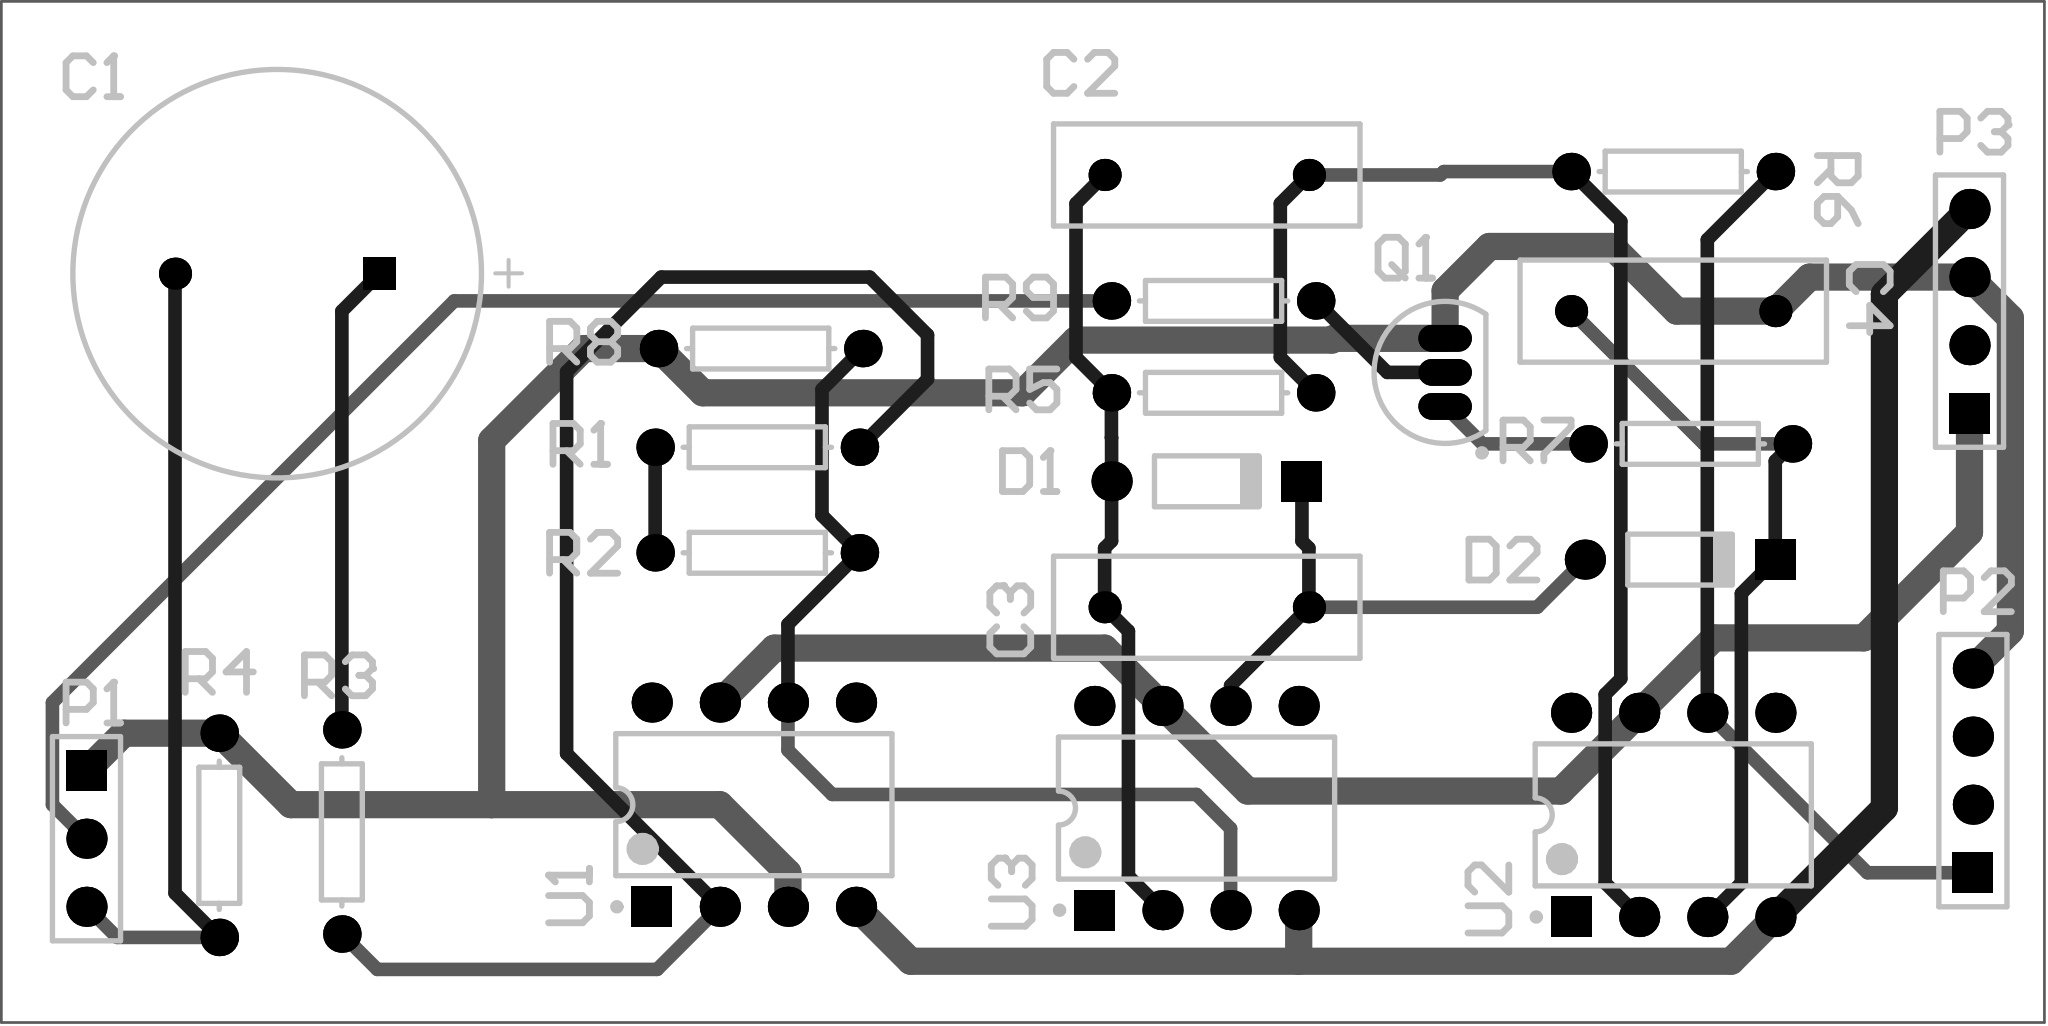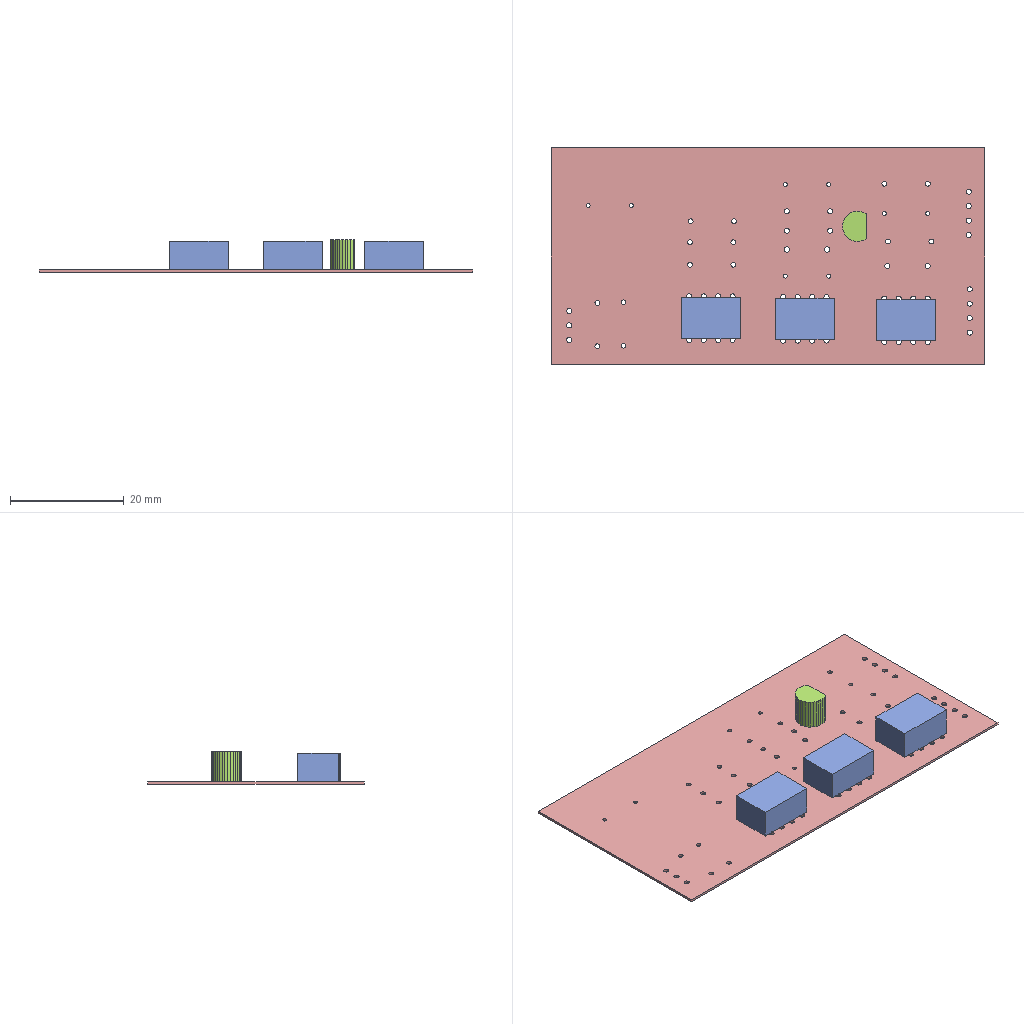Circuit board layout | Altium Designer | box 76.2 x 38.1 x 5.7 mm
Layer stack:
# Altium Designer layer stack of  (unit mm; dielectric type: 0 none, 1 core, 2 prepreg, 3 surface material)
index,name,kind,layer,copper_thickness_mm,dielectric_type,dielectric_thickness_mm,dielectric_material,dielectric_constant
0,Top Paste,other,,,,,,
1,Top Overlay,other,,,,,,
2,Top Solder,dielectric,,,3,0.0102,Solder Resist,3.5
3,Top Layer,copper,Top Layer,0.0356,,,,
4,Dielectric 1,dielectric,,,0,0.32,FR-4,4.8
5,Bottom Layer,copper,Bottom Layer,0.0356,,,,
6,Bottom Solder,dielectric,,,3,0.0102,Solder Resist,3.5
7,Bottom Overlay,other,,,,,,
8,Bottom Paste,other,,,,,,
# drill layer pairs: low layer,high layer
drill_pair,Top Layer,Bottom Layer
Part placement:
Designator,Comment,Layer,Footprint,Center-X(mm),Center-Y(mm),Rotation
U3,UA741AN,TopLayer,DIP-8,69.977,33.401,90
U2,UA741AN,TopLayer,DIP-8,87.757,33.147,90
U1,UA741AN,TopLayer,DIP-8,53.467,33.528,90
R9,Res1,TopLayer,AXIAL-0.3,70.612,52.324,180
R8,Res1,TopLayer,AXIAL-0.3,53.721,50.546,360
R7,Res1,TopLayer,AXIAL-0.3,88.392,46.99,180
R6,Res1,TopLayer,AXIAL-0.3,87.757,57.15,360
R5,Res1,TopLayer,AXIAL-0.3,70.612,48.895,360
R4,Res1,TopLayer,AXIAL-0.3,33.528,32.385,270
R3,Res1,TopLayer,AXIAL-0.3,38.1,32.512,270
R2,Res1,TopLayer,AXIAL-0.3,53.594,42.926,360
R1,Res1,TopLayer,AXIAL-0.3,53.594,46.863,180
Q1,NPN,TopLayer,TO-226-AA,79.248,49.657,0
P3,Header 4,TopLayer,HDR1X4,98.806,51.943,90
P2,Header 4,TopLayer,HDR1X4,98.933,34.798,90
P1,Header 3,TopLayer,HDR1X3,28.575,32.258,270
D2,Diode 1N914,TopLayer,DO-35,88.011,42.672,360
D1,Diode 1N914,TopLayer,DO-35,70.358,45.593,360
C4,Cap,TopLayer,RAD-0.3,87.757,51.943,360
C3,Cap,TopLayer,RAD-0.3,70.358,40.894,180
C2,Cap,TopLayer,RAD-0.3,70.358,57.023,180
C1,Cap Pol1,TopLayer,RB7.6-15,35.687,53.34,0
Pad and via stacks:
# Altium Designer via and pad stacks of  (unit mm). Each distinct definition once, with the count of objects using it.
# via: kind,start_layer,end_layer,hole_mm,diameter_mm,mode(0 simple;1 top-mid-bottom;2 full stack),diameter_per_layer,count,example_net
# pad: kind,layer,hole_mm,hole_type(0 round;1 square;2 slot),plating,top_size,top_shape(1 round;2 rect;3 octagon;9 rounded rect),mid_size,bottom_size,mode,footprint,size_per_layer,count,example
pad,Multi-Layer,0.7,0,plated,1.2x1.2,1,1.2x1.2,1.2x1.2,0,RAD-0.3,,6,C2.2
pad,Multi-Layer,0.85,0,plated,1.4x1.4,1,1.4x1.4,1.4x1.4,0,AXIAL-0.3,,18,R6.2
pad,Multi-Layer,0.9,0,plated,1.5x1.5,2,1.5x1.5,1.5x1.5,0,DO-35,,2,D1.2
pad,Multi-Layer,0.9,0,plated,1.5x1.5,1,1.5x1.5,1.5x1.5,0,DO-35,,2,D1.1
pad,Multi-Layer,0.9,0,plated,1.5x1.5,2,1.5x1.5,1.5x1.5,0,DIP-8,,3,U2.1
pad,Multi-Layer,0.9,0,plated,1.5x1.5,1,1.5x1.5,1.5x1.5,0,DIP-8,,21,U2.2
pad,Multi-Layer,0.9,0,plated,1.5x1.5,1,1.5x1.5,1.5x1.5,0,HDR1X4,,6,P2.4
pad,Multi-Layer,0.9,0,plated,1.5x1.5,2,1.5x1.5,1.5x1.5,0,HDR1X4,,2,P2.1
pad,Multi-Layer,0.9,0,plated,2x1,1,2x1,2x1,0,TO-226-AA,,3,Q1.1
pad,Multi-Layer,0.7,0,plated,1.2x1.2,2,1.2x1.2,1.2x1.2,0,RB7.6-15,,1,C1.1
pad,Multi-Layer,0.7,0,plated,1.2x1.2,1,1.2x1.2,1.2x1.2,0,RB7.6-15,,1,C1.2
pad,Multi-Layer,0.9,0,plated,1.5x1.5,2,1.5x1.5,1.5x1.5,0,HDR1X3,,1,P1.1
pad,Multi-Layer,0.9,0,plated,1.5x1.5,1,1.5x1.5,1.5x1.5,0,HDR1X3,,2,P1.2
Design rules, without the lines most boards share:
# Altium Designer design rules of  (exported by Altium Designer, unit mm)
# columns: name | kind | enabled | priority | scope1 | scope2 | descriptor | typed fields (field=value)
HoleToHoleClearance | 52 | enabled | 1 | All | All | Hole To Hole Clearance (Gap=10mil) (All),(All) | gap=0.254
DiffPairsRouting | 51 | enabled | 1 | All | All | Differential Pairs Uncoupled Length using the Gap Constraints (Min=10mil) (Max=10mil) (Prefered=10mil)  and Width Constraints (Min=15mil) (Max=15mil) (Prefered=15mil) (All) |
SolderMaskExpansion | 13 | enabled | 1 | All | All | Solder Mask Expansion (Expansion =4mil) (All) | expansion=0.1016
PasteMaskExpansion | 14 | enabled | 1 | All | All | Paste Mask Expansion (Expansion =0mil) (All) | expansion=0
RoutingVias | 11 | enabled | 1 | All | All | Routing Via (MinHoleWidth=28mil) (MaxHoleWidth=28mil) (PreferredHoleWidth=28mil) (MinWidth=50mil) (MaxWidth=50mil) (PreferedWidth=50mil) (All) | via_min_hole=0.7112 via_max_hole=0.7112 via_preferred_diameter=1.27 via_preferred_hole=0.7112
Width | 2 | enabled | 1 | All | All | Width Constraint (Min=20mil) (Max=40mil) (Preferred=20mil) (All) |
PolygonConnect | 20 | enabled | 1 | All | All | Polygon Connect Rule(Relief Connect )(Conductor Width=10mil) (Relief Angle=90 Angle) (Entries=4) (Air Gap Width=10mil) (All),(All) | connect_style(0=relief,1=direct,2=none)=0 relief_conductor_width=0.254 relief_entries=4
PlaneConnect | 6 | enabled | 1 | All | All | Power Plane Connect Rule(Relief Connect )(Expansion=20mil) (Conductor Width=10mil) (Air Gap=10mil) (Entries=4) (All) | relief_conductor_width=0.254 relief_entries=4 relief_expansion=0.508
Clearance | 0 | enabled | 1 | All | All | Clearance Constraint (Gap=10mil) (All),(All) | gap=0.254